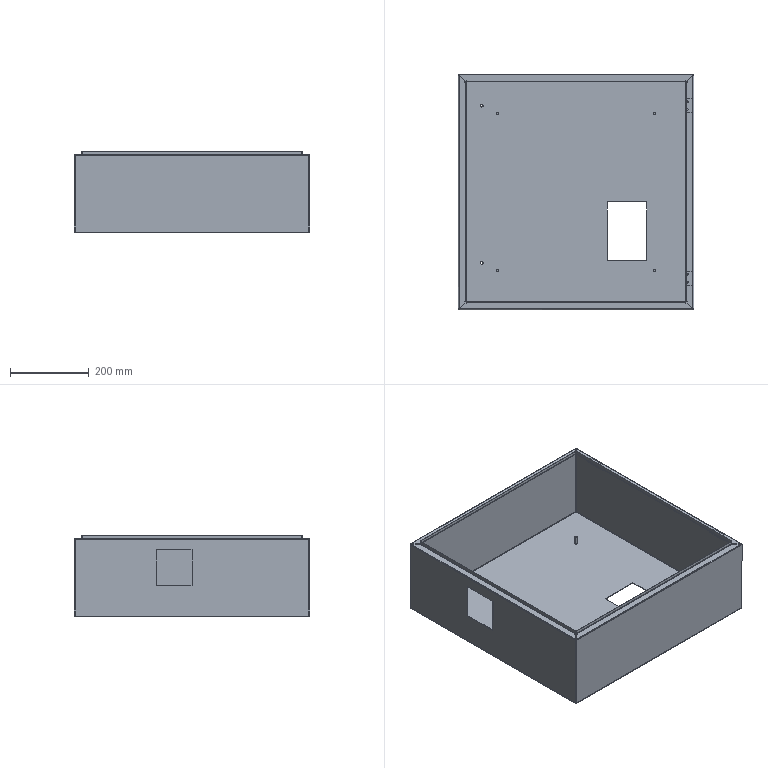Part | SolidWorks | features LocalLPattern 1, ReferencePattern 1 | 3 solids | 186 faces | box 600 x 600 x 208.5 mm | volume 1307519 mm3 | plane 122 | cylinder 48 | spline 16 | commonest cylinder face diameters 1.473 x14 4.473 x12 4.5 x8 6 x8 7 x4 5.473 x2